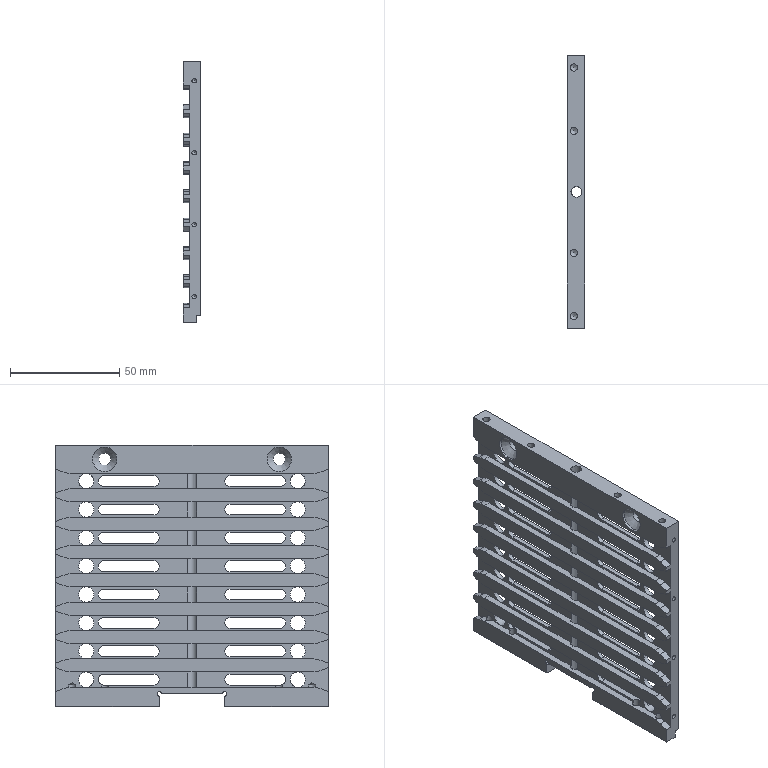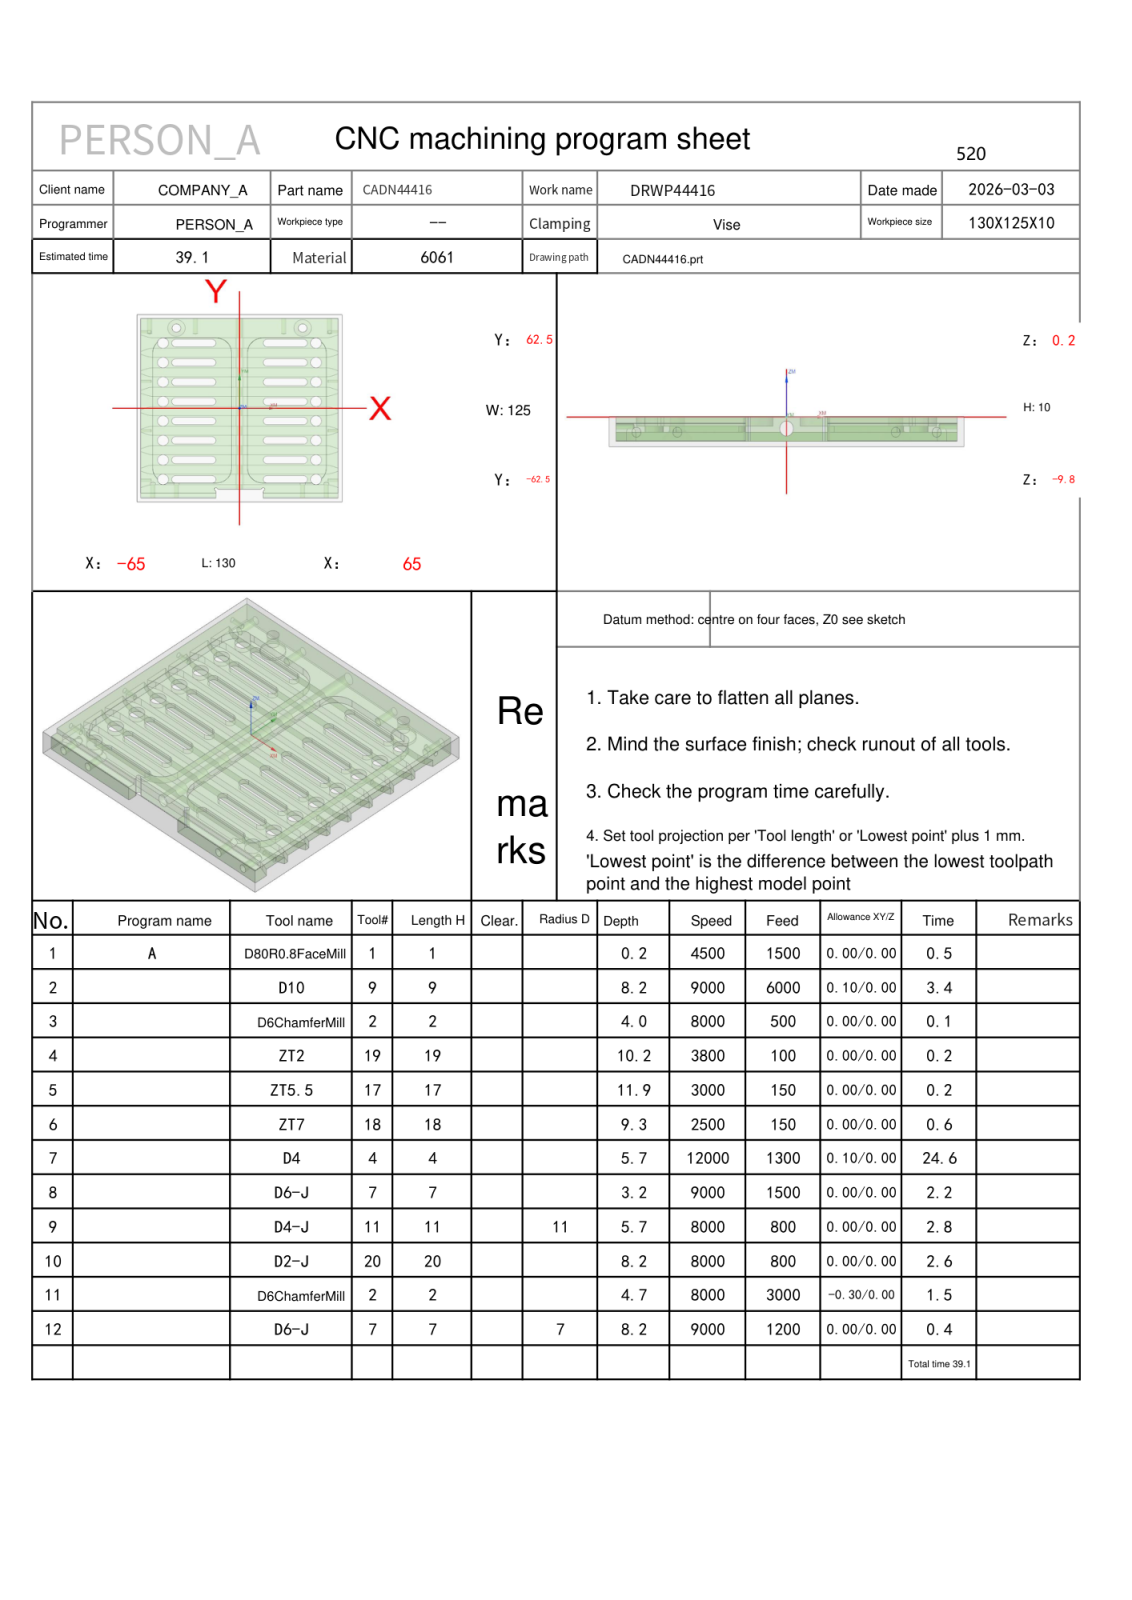NC program | NX | posted by the shop | part box 8 x 125 x 120 mm
Lines 1 to 825 of 11100:
%
O0001
(Machine time: 41.28 MIN)
(===Total Tool:10===)
(T1=D80R0.8 FaceMill D=80.  R=0.8  D-  H01 Z=0.    )
(T9=D10     D=10.  R=0.   D-  H09 Z=-8.   )
(T2=D6ChamferMill   D=6.   R=0.   D-  H02 Z=-4.5  )
(T19=ZT2    D=2.   DR_a=118 D-  H19 Z=-10.  )
(T17=ZT5.5  D=5.5  DR_a=118 D-  H17 Z=-11.65)
(T18=ZT7    D=7.   DR_a=118 D-  H18 Z=-9.1  )
(T4=D4      D=4.   R=0.   D-  H04 Z=-5.5  )
(T7=D6-J    D=6.   R=0.   D7  H07 Z=-8.   )
(T11=D4-J   D=4.   R=0.   D11 H11 Z=-5.5  )
(T20=D2-J   D=2.   R=0.   D-  H20 Z=-8.   )
G80 G90 G17 G49 G40
G91 G28 Z0
M01
N1 T01 M06
(D80R0.8 FaceMill  D=80. R=0.8 H=01 ce=0.00 di=0.00)
G00 G90 G54 X-107.5 Y50. M03 S4500
G43 H01 Z30.
M08
Z2.
G01 Z0.0 F1500.
X-102.5
X102.5
Y0.0
X-102.5
Y-50.
X102.5
X107.5
Z2.
G00 Z30.
G91 G28 Z0.0
M05
M09
G91 G28 Z0.0
M01
N2 T09 M06
(D10  D=10. R=0. H=09 ce=0.10 di=0.00)
G00 G90 G54 X0.0 Y65.1 M03 S8000
G43 H09 Z30.
M08
Z.5
G01 X62.5 Z.409 F6000.
G02 X67.6 Y60. Z.397 I0.0 J-5.1
G01 Y-60. Z.222
G02 X62.5 Y-65.1 Z.21 I-5.1 J0.0
G01 X15. Z.141
G02 X9.9 Y-60. Z.129 I0.0 J5.1
G01 Y-59.1 Z.128
X-9.9 Z.099
Y-60. Z.098
G02 X-15. Y-65.1 Z.086 I-5.1 J0.0
G01 X-62.5 Z.017
G02 X-67.6 Y-60. Z.005 I0.0 J5.1
G01 Y60. Z-.17
G02 X-62.5 Y65.1 Z-.182 I5.1 J0.0
G01 X62.5 Z-.364
G02 X67.6 Y60. Z-.376 I0.0 J-5.1
G01 Y-60. Z-.551
G02 X62.5 Y-65.1 Z-.562 I-5.1 J0.0
G01 X15. Z-.632
G02 X9.9 Y-60. Z-.643 I0.0 J5.1
G01 Y-59.1 Z-.645
X-9.9 Z-.674
Y-60. Z-.675
G02 X-15. Y-65.1 Z-.687 I-5.1 J0.0
G01 X-62.5 Z-.756
G02 X-67.6 Y-60. Z-.768 I0.0 J5.1
G01 Y60. Z-.943
G02 X-62.5 Y65.1 Z-.954 I5.1 J0.0
G01 X62.5 Z-1.137
G02 X67.6 Y60. Z-1.148 I0.0 J-5.1
G01 Y-60. Z-1.323
G02 X62.5 Y-65.1 Z-1.335 I-5.1 J0.0
G01 X15. Z-1.404
G02 X9.9 Y-60. Z-1.416 I0.0 J5.1
G01 Y-59.1 Z-1.417
X-9.9 Z-1.446
Y-60. Z-1.448
G02 X-15. Y-65.1 Z-1.459 I-5.1 J0.0
G01 X-62.5 Z-1.529
G02 X-67.6 Y-60. Z-1.54 I0.0 J5.1
G01 Y60. Z-1.715
G02 X-62.5 Y65.1 Z-1.727 I5.1 J0.0
G01 X62.5 Z-1.909
G02 X67.6 Y60. Z-1.921 I0.0 J-5.1
G01 Y-60. Z-2.096
G02 X62.5 Y-65.1 Z-2.108 I-5.1 J0.0
G01 X15. Z-2.177
G02 X9.9 Y-60. Z-2.189 I0.0 J5.1
G01 Y-59.1 Z-2.19
X-9.9 Z-2.219
Y-60. Z-2.22
G02 X-15. Y-65.1 Z-2.232 I-5.1 J0.0
G01 X-62.5 Z-2.301
G02 X-67.6 Y-60. Z-2.313 I0.0 J5.1
G01 Y60. Z-2.488
G02 X-62.5 Y65.1 Z-2.5 I5.1 J0.0
G01 X62.5 Z-2.682
G02 X67.6 Y60. Z-2.694 I0.0 J-5.1
G01 Y-60. Z-2.869
G02 X62.5 Y-65.1 Z-2.881 I-5.1 J0.0
G01 X15. Z-2.95
G02 X9.9 Y-60. Z-2.962 I0.0 J5.1
G01 Y-59.1 Z-2.963
X-9.9 Z-2.992
Y-60. Z-2.993
G02 X-15. Y-65.1 Z-3.005 I-5.1 J0.0
G01 X-62.5 Z-3.074
G02 X-67.6 Y-60. Z-3.086 I0.0 J5.1
G01 Y60. Z-3.261
G02 X-62.5 Y65.1 Z-3.272 I5.1 J0.0
G01 X62.5 Z-3.455
G02 X67.6 Y60. Z-3.467 I0.0 J-5.1
G01 Y-60. Z-3.642
G02 X62.5 Y-65.1 Z-3.653 I-5.1 J0.0
G01 X15. Z-3.723
G02 X9.9 Y-60. Z-3.734 I0.0 J5.1
G01 Y-59.1 Z-3.736
X-9.9 Z-3.764
Y-60. Z-3.766
G02 X-15. Y-65.1 Z-3.777 I-5.1 J0.0
G01 X-62.5 Z-3.847
G02 X-67.6 Y-60. Z-3.858 I0.0 J5.1
G01 Y60. Z-4.033
G02 X-62.5 Y65.1 Z-4.045 I5.1 J0.0
G01 X62.5 Z-4.228
G02 X67.6 Y60. Z-4.239 I0.0 J-5.1
G01 Y-60. Z-4.414
G02 X62.5 Y-65.1 Z-4.426 I-5.1 J0.0
G01 X15. Z-4.495
G02 X9.9 Y-60. Z-4.507 I0.0 J5.1
G01 Y-59.1 Z-4.508
X-9.9 Z-4.537
Y-60. Z-4.538
G02 X-15. Y-65.1 Z-4.55 I-5.1 J0.0
G01 X-62.5 Z-4.619
G02 X-67.6 Y-60. Z-4.631 I0.0 J5.1
G01 Y60. Z-4.806
G02 X-62.5 Y65.1 Z-4.818 I5.1 J0.0
G01 X62.5 Z-5.
G02 X67.6 Y60. Z-5.012 I0.0 J-5.1
G01 Y-60. Z-5.187
G02 X62.5 Y-65.1 Z-5.199 I-5.1 J0.0
G01 X15. Z-5.268
G02 X9.9 Y-60. Z-5.28 I0.0 J5.1
G01 Y-59.1 Z-5.281
X-9.9 Z-5.31
Y-60. Z-5.311
G02 X-15. Y-65.1 Z-5.323 I-5.1 J0.0
G01 X-62.5 Z-5.392
G02 X-67.6 Y-60. Z-5.404 I0.0 J5.1
G01 Y60. Z-5.579
G02 X-62.5 Y65.1 Z-5.591 I5.1 J0.0
G01 X62.5 Z-5.773
G02 X67.6 Y60. Z-5.785 I0.0 J-5.1
G01 Y-60. Z-5.96
G02 X62.5 Y-65.1 Z-5.971 I-5.1 J0.0
G01 X15. Z-6.041
G02 X9.9 Y-60. Z-6.052 I0.0 J5.1
G01 Y-59.1 Z-6.054
X-9.9 Z-6.083
Y-60. Z-6.084
G02 X-15. Y-65.1 Z-6.096 I-5.1 J0.0
G01 X-62.5 Z-6.165
G02 X-67.6 Y-60. Z-6.177 I0.0 J5.1
G01 Y60. Z-6.352
G02 X-62.5 Y65.1 Z-6.363 I5.1 J0.0
G01 X62.5 Z-6.546
G02 X67.6 Y60. Z-6.557 I0.0 J-5.1
G01 Y-60. Z-6.732
G02 X62.5 Y-65.1 Z-6.744 I-5.1 J0.0
G01 X15. Z-6.813
G02 X9.9 Y-60. Z-6.825 I0.0 J5.1
G01 Y-59.1 Z-6.826
X-9.9 Z-6.855
Y-60. Z-6.857
G02 X-15. Y-65.1 Z-6.868 I-5.1 J0.0
G01 X-62.5 Z-6.938
G02 X-67.6 Y-60. Z-6.949 I0.0 J5.1
G01 Y60. Z-7.124
G02 X-62.5 Y65.1 Z-7.136 I5.1 J0.0
G01 X62.5 Z-7.318
G02 X67.6 Y60. Z-7.33 I0.0 J-5.1
G01 Y-60. Z-7.505
G02 X62.5 Y-65.1 Z-7.517 I-5.1 J0.0
G01 X15. Z-7.586
G02 X9.9 Y-60. Z-7.598 I0.0 J5.1
G01 Y-59.1 Z-7.599
X-9.9 Z-7.628
Y-60. Z-7.629
G02 X-15. Y-65.1 Z-7.641 I-5.1 J0.0
G01 X-62.5 Z-7.71
G02 X-67.6 Y-60. Z-7.722 I0.0 J5.1
G01 Y60. Z-7.897
G02 X-62.5 Y65.1 Z-7.909 I5.1 J0.0
G01 X0.0 Z-8.
X62.5
G02 X67.6 Y60. I0.0 J-5.1
G01 Y-60.
G02 X62.5 Y-65.1 I-5.1 J0.0
G01 X15.
G02 X9.9 Y-60. I0.0 J5.1
G01 Y-59.1
X-9.9
Y-60.
G02 X-15. Y-65.1 I-5.1 J0.0
G01 X-62.5
G02 X-67.6 Y-60. I0.0 J5.1
G01 Y60.
G02 X-62.5 Y65.1 I5.1 J0.0
G01 X0.0
X.5
Z-7.
G00 Z30.
G00 G90 X28.6 Y-16.548 M03 S9000
Z30.
Z.5
G01 Y-26.4 Z.242 F4000.
X31.4 Z.169
Y-1.5 Z-.483
Y23.4
X28.6
Y-26.4
X31.4
Y-1.5
X35.9
Y27.9
X24.1
Y-30.9
X35.9
Y-1.5
X42.9
Y34.9
X17.1
Y-37.9
X42.9
Y-1.5
X49.9
Y37.
G03 X48.394 Y40.534 I-4.9 J0.0
G02 X47.51 Y41.662 I3.533 J3.678
X47.209 Y41.653 I-.302 J5.091
X46.082 Y41.779 I0.0 J5.1
G03 X45. Y41.9 I-1.082 J-4.779
G01 X15.
G03 X10.1 Y37. I0.0 J-4.9
G01 Y-40.
G03 X15. Y-44.9 I4.9 J0.0
G01 X45.
G03 X45.49 Y-44.875 I0.0 J4.9
G02 X46. Y-44.85 I.51 J-5.074
X47.348 Y-45.031 I0.0 J-5.1
X48.422 Y-43.507 I4.635 J-2.127
G03 X49.9 Y-40. I-3.422 J3.507
G01 Y-1.5
Y-1.
Z.017
G00 Z.5
X28.6 Y-16.548
Z.017
G01 Y-26.4 Z-.241
X31.4 Z-.315
Y-1.5 Z-.967
Y23.4
X28.6
Y-26.4
X31.4
Y-1.5
X35.9
Y27.9
X24.1
Y-30.9
X35.9
Y-1.5
X42.9
Y34.9
X17.1
Y-37.9
X42.9
Y-1.5
X49.9
Y37.
G03 X48.394 Y40.534 I-4.9 J0.0
G02 X47.51 Y41.662 I3.533 J3.678
X47.209 Y41.653 I-.302 J5.091
X46.082 Y41.779 I0.0 J5.1
G03 X45. Y41.9 I-1.082 J-4.779
G01 X15.
G03 X10.1 Y37. I0.0 J-4.9
G01 Y-40.
G03 X15. Y-44.9 I4.9 J0.0
G01 X45.
G03 X45.49 Y-44.875 I0.0 J4.9
G02 X46. Y-44.85 I.51 J-5.074
X47.348 Y-45.031 I0.0 J-5.1
X48.422 Y-43.507 I4.635 J-2.127
G03 X49.9 Y-40. I-3.422 J3.507
G01 Y-1.5
Y-1.
Z-.467
G00 Z.017
X28.6 Y-16.548
Z-.467
G01 Y-26.4 Z-.725
X31.4 Z-.798
Y-1.5 Z-1.45
Y23.4
X28.6
Y-26.4
X31.4
Y-1.5
X35.9
Y27.9
X24.1
Y-30.9
X35.9
Y-1.5
X42.9
Y34.9
X17.1
Y-37.9
X42.9
Y-1.5
X49.9
Y37.
G03 X48.394 Y40.534 I-4.9 J0.0
G02 X47.51 Y41.662 I3.533 J3.678
X47.209 Y41.653 I-.302 J5.091
X46.082 Y41.779 I0.0 J5.1
G03 X45. Y41.9 I-1.082 J-4.779
G01 X15.
G03 X10.1 Y37. I0.0 J-4.9
G01 Y-40.
G03 X15. Y-44.9 I4.9 J0.0
G01 X45.
G03 X45.49 Y-44.875 I0.0 J4.9
G02 X46. Y-44.85 I.51 J-5.074
X47.348 Y-45.031 I0.0 J-5.1
X48.422 Y-43.507 I4.635 J-2.127
G03 X49.9 Y-40. I-3.422 J3.507
G01 Y-1.5
Y-1.
Z-.95
G00 Z-.467
X28.6 Y-16.548
Z-.95
G01 Y-26.4 Z-1.208
X31.4 Z-1.281
Y-1.5 Z-1.933
Y23.4
X28.6
Y-26.4
X31.4
Y-1.5
X35.9
Y27.9
X24.1
Y-30.9
X35.9
Y-1.5
X42.9
Y34.9
X17.1
Y-37.9
X42.9
Y-1.5
X49.9
Y37.
G03 X48.394 Y40.534 I-4.9 J0.0
G02 X47.51 Y41.662 I3.533 J3.678
X47.209 Y41.653 I-.302 J5.091
X46.082 Y41.779 I0.0 J5.1
G03 X45. Y41.9 I-1.082 J-4.779
G01 X15.
G03 X10.1 Y37. I0.0 J-4.9
G01 Y-40.
G03 X15. Y-44.9 I4.9 J0.0
G01 X45.
G03 X45.49 Y-44.875 I0.0 J4.9
G02 X46. Y-44.85 I.51 J-5.074
X47.348 Y-45.031 I0.0 J-5.1
X48.422 Y-43.507 I4.635 J-2.127
G03 X49.9 Y-40. I-3.422 J3.507
G01 Y-1.5
Y-1.
Z-1.433
G00 Z-.95
X28.6 Y-16.548
Z-1.433
G01 Y-26.4 Z-1.691
X31.4 Z-1.765
Y-1.5 Z-2.417
Y23.4
X28.6
Y-26.4
X31.4
Y-1.5
X35.9
Y27.9
X24.1
Y-30.9
X35.9
Y-1.5
X42.9
Y34.9
X17.1
Y-37.9
X42.9
Y-1.5
X49.9
Y37.
G03 X48.394 Y40.534 I-4.9 J0.0
G02 X47.51 Y41.662 I3.533 J3.678
X47.209 Y41.653 I-.302 J5.091
X46.082 Y41.779 I0.0 J5.1
G03 X45. Y41.9 I-1.082 J-4.779
G01 X15.
G03 X10.1 Y37. I0.0 J-4.9
G01 Y-40.
G03 X15. Y-44.9 I4.9 J0.0
G01 X45.
G03 X45.49 Y-44.875 I0.0 J4.9
G02 X46. Y-44.85 I.51 J-5.074
X47.348 Y-45.031 I0.0 J-5.1
X48.422 Y-43.507 I4.635 J-2.127
G03 X49.9 Y-40. I-3.422 J3.507
G01 Y-1.5
Y-1.
Z-1.917
G00 Z-1.433
X28.6 Y-16.548
Z-1.917
G01 Y-26.4 Z-2.175
X31.4 Z-2.248
Y-1.5 Z-2.9
Y23.4
X28.6
Y-26.4
X31.4
Y-1.5
X35.9
Y27.9
X24.1
Y-30.9
X35.9
Y-1.5
X42.9
Y34.9
X17.1
Y-37.9
X42.9
Y-1.5
X49.9
Y37.
G03 X48.394 Y40.534 I-4.9 J0.0
G02 X47.51 Y41.662 I3.533 J3.678
X47.209 Y41.653 I-.302 J5.091
X46.082 Y41.779 I0.0 J5.1
G03 X45. Y41.9 I-1.082 J-4.779
G01 X15.
G03 X10.1 Y37. I0.0 J-4.9
G01 Y-40.
G03 X15. Y-44.9 I4.9 J0.0
G01 X45.
G03 X45.49 Y-44.875 I0.0 J4.9
G02 X46. Y-44.85 I.51 J-5.074
X47.348 Y-45.031 I0.0 J-5.1
X48.422 Y-43.507 I4.635 J-2.127
G03 X49.9 Y-40. I-3.422 J3.507
G01 Y-1.5
Y-1.
Z-2.4
G00 Z30.
X-28.6 Y13.548
Z.5
G01 Y23.4 Z.242
X-31.4 Z.169
Y-1.5 Z-.483
Y-26.4
X-28.6
Y23.4
X-31.4
Y-1.5
X-35.9
Y-30.9
X-24.1
Y27.9
X-35.9
Y-1.5
X-42.9
Y-37.9
X-17.1
Y34.9
X-42.9
Y-1.5
X-49.9
Y-40.
G03 X-48.422 Y-43.507 I4.9 J0.0
G02 X-47.348 Y-45.031 I-3.561 J-3.65
X-46. Y-44.85 I1.347 J-4.919
X-45.49 Y-44.875 I0.0 J-5.1
G03 X-45. Y-44.9 I.49 J4.875
G01 X-15.
G03 X-10.1 Y-40. I0.0 J4.9
G01 Y37.
G03 X-15. Y41.9 I-4.9 J0.0
G01 X-45.
G03 X-46.082 Y41.779 I0.0 J-4.9
G02 X-47.209 Y41.653 I-1.126 J4.974
X-47.51 Y41.662 I0.0 J5.1
X-48.394 Y40.534 I-4.416 J2.551
G03 X-49.9 Y37. I3.394 J-3.534
G01 Y-1.5
Y-2.
Z.017
G00 Z.5
X-28.6 Y13.548
Z.017
G01 Y23.4 Z-.241
X-31.4 Z-.315
Y-1.5 Z-.967
Y-26.4
X-28.6
Y23.4
X-31.4
Y-1.5
X-35.9
Y-30.9
X-24.1
Y27.9
X-35.9
Y-1.5
X-42.9
Y-37.9
X-17.1
Y34.9
X-42.9
Y-1.5
X-49.9
Y-40.
G03 X-48.422 Y-43.507 I4.9 J0.0
G02 X-47.348 Y-45.031 I-3.561 J-3.65
X-46. Y-44.85 I1.347 J-4.919
X-45.49 Y-44.875 I0.0 J-5.1
G03 X-45. Y-44.9 I.49 J4.875
G01 X-15.
G03 X-10.1 Y-40. I0.0 J4.9
G01 Y37.
G03 X-15. Y41.9 I-4.9 J0.0
G01 X-45.
G03 X-46.082 Y41.779 I0.0 J-4.9
G02 X-47.209 Y41.653 I-1.126 J4.974
X-47.51 Y41.662 I0.0 J5.1
X-48.394 Y40.534 I-4.416 J2.551
G03 X-49.9 Y37. I3.394 J-3.534
G01 Y-1.5
Y-2.
Z-.467
G00 Z.017
X-28.6 Y13.548
Z-.467
G01 Y23.4 Z-.725
X-31.4 Z-.798
Y-1.5 Z-1.45
Y-26.4
X-28.6
Y23.4
X-31.4
Y-1.5
X-35.9
Y-30.9
X-24.1
Y27.9
X-35.9
Y-1.5
X-42.9
Y-37.9
X-17.1
Y34.9
X-42.9
Y-1.5
X-49.9
Y-40.
G03 X-48.422 Y-43.507 I4.9 J0.0
G02 X-47.348 Y-45.031 I-3.561 J-3.65
X-46. Y-44.85 I1.347 J-4.919
X-45.49 Y-44.875 I0.0 J-5.1
G03 X-45. Y-44.9 I.49 J4.875
G01 X-15.
G03 X-10.1 Y-40. I0.0 J4.9
G01 Y37.
G03 X-15. Y41.9 I-4.9 J0.0
G01 X-45.
G03 X-46.082 Y41.779 I0.0 J-4.9
G02 X-47.209 Y41.653 I-1.126 J4.974
X-47.51 Y41.662 I0.0 J5.1
X-48.394 Y40.534 I-4.416 J2.551
G03 X-49.9 Y37. I3.394 J-3.534
G01 Y-1.5
Y-2.
Z-.95
G00 Z-.467
X-28.6 Y13.548
Z-.95
G01 Y23.4 Z-1.208
X-31.4 Z-1.281
Y-1.5 Z-1.933
Y-26.4
X-28.6
Y23.4
X-31.4
Y-1.5
X-35.9
Y-30.9
X-24.1
Y27.9
X-35.9
Y-1.5
X-42.9
Y-37.9
X-17.1
Y34.9
X-42.9
Y-1.5
X-49.9
Y-40.
G03 X-48.422 Y-43.507 I4.9 J0.0
G02 X-47.348 Y-45.031 I-3.561 J-3.65
X-46. Y-44.85 I1.347 J-4.919
X-45.49 Y-44.875 I0.0 J-5.1
G03 X-45. Y-44.9 I.49 J4.875
G01 X-15.
G03 X-10.1 Y-40. I0.0 J4.9
G01 Y37.
G03 X-15. Y41.9 I-4.9 J0.0
G01 X-45.
G03 X-46.082 Y41.779 I0.0 J-4.9
G02 X-47.209 Y41.653 I-1.126 J4.974
X-47.51 Y41.662 I0.0 J5.1
X-48.394 Y40.534 I-4.416 J2.551
G03 X-49.9 Y37. I3.394 J-3.534
G01 Y-1.5
Y-2.
Z-1.433
G00 Z-.95
X-28.6 Y13.548
Z-1.433
G01 Y23.4 Z-1.691
X-31.4 Z-1.765
Y-1.5 Z-2.417
Y-26.4
X-28.6
Y23.4
X-31.4
Y-1.5
X-35.9
Y-30.9
X-24.1
Y27.9
X-35.9
Y-1.5
X-42.9
Y-37.9
X-17.1
Y34.9
X-42.9
Y-1.5
X-49.9
Y-40.
G03 X-48.422 Y-43.507 I4.9 J0.0
G02 X-47.348 Y-45.031 I-3.561 J-3.65
X-46. Y-44.85 I1.347 J-4.919
X-45.49 Y-44.875 I0.0 J-5.1
G03 X-45. Y-44.9 I.49 J4.875
G01 X-15.
G03 X-10.1 Y-40. I0.0 J4.9
G01 Y37.
G03 X-15. Y41.9 I-4.9 J0.0
G01 X-45.
G03 X-46.082 Y41.779 I0.0 J-4.9
G02 X-47.209 Y41.653 I-1.126 J4.974
X-47.51 Y41.662 I0.0 J5.1
X-48.394 Y40.534 I-4.416 J2.551
G03 X-49.9 Y37. I3.394 J-3.534
G01 Y-1.5
Y-2.
Z-1.917
G00 Z-1.433
X-28.6 Y13.548
Z-1.917
G01 Y23.4 Z-2.175
X-31.4 Z-2.248
Y-1.5 Z-2.9
Y-26.4
X-28.6
Y23.4
X-31.4
Y-1.5
X-35.9
Y-30.9
X-24.1
Y27.9
X-35.9
Y-1.5
X-42.9
Y-37.9
X-17.1
Y34.9
X-42.9
Y-1.5
X-49.9
Y-40.
G03 X-48.422 Y-43.507 I4.9 J0.0
G02 X-47.348 Y-45.031 I-3.561 J-3.65
X-46. Y-44.85 I1.347 J-4.919
X-45.49 Y-44.875 I0.0 J-5.1
G03 X-45. Y-44.9 I.49 J4.875
G01 X-15.
G03 X-10.1 Y-40. I0.0 J4.9
G01 Y37.
G03 X-15. Y41.9 I-4.9 J0.0
G01 X-45.
G03 X-46.082 Y41.779 I0.0 J-4.9
G02 X-47.209 Y41.653 I-1.126 J4.974
X-47.51 Y41.662 I0.0 J5.1
X-48.394 Y40.534 I-4.416 J2.551
G03 X-49.9 Y37. I3.394 J-3.534
G01 Y-1.5
Y-2.
Z-2.4
G00 Z30.
G91 G28 Z0.0
M05
M09
G91 G28 Z0.0
M01
N3 T02 M06
(D6ChamferMill  D=6. R=0. H=02 ce=0.00 di=0.10)
G00 G90 G54 X-15. Y-54. M03 S3000
G43 H02 Z30.
M08
G98 G81 X-15. Y-54. Z-1.55 R1. F200.
X15.
G80
G00 Z30.
G00 G90 X48.5 Y-34.5 M03 S8000
Z30.
G98 G81 X48.5 Y-34.5 Z-3.8 R-2. F500.
Y-21.5
Y-8.5
Y4.5
Y17.5
Y30.5
X40. Y53.5 Z-.8 R1.
X-40.
X-48.5 Y30.5 Z-3.8 R-2.
Y17.5
Y4.5
Y-8.5
Y-21.5
Y-34.5
G80
G00 Z30.
G91 G28 Z0.0
M05
M09
G91 G28 Z0.0
M01
N4 T19 M06
(ZT2 D=2. DR_a=118 H=19)
G00 G90 G54 X-15. Y-54. M03 S3800
G43 H19 Z30.
M08
G98 G83 X-15. Y-54. Z-10. R1. F100. Q1.5
X15.
G80
G00 Z30.
G91 G28 Z0.0
M05
M09
G91 G28 Z0.0
M01
N5 T17 M06
(ZT5.5 D=5.5 DR_a=118 H=17)
G00 G90 G54 X40. Y53.5 M03 S3000
G43 H17 Z30.
M08
G98 G83 X40. Y53.5 Z-11.652 R1. F150. Q3.
X-40.
G80
G00 Z30.
G91 G28 Z0.0
M05
M09
G91 G28 Z0.0
M01
N6 T18 M06
(ZT7 D=7. DR_a=118 H=18)
G00 G90 G54 X-48.5 Y-34.5 M03 S2500
G43 H18 Z30.
M08
G98 G83 X-48.5 Y-34.5 Z-9.103 R-2. F150. Q3.
Y-21.5
Y-8.5
Y4.5
Y17.5
Y30.5
X48.5
Y17.5
Y4.5
Y-8.5
Y-21.5
Y-34.5
G80
G00 Z30.
G91 G28 Z0.0
M05
M09
G91 G28 Z0.0
M01